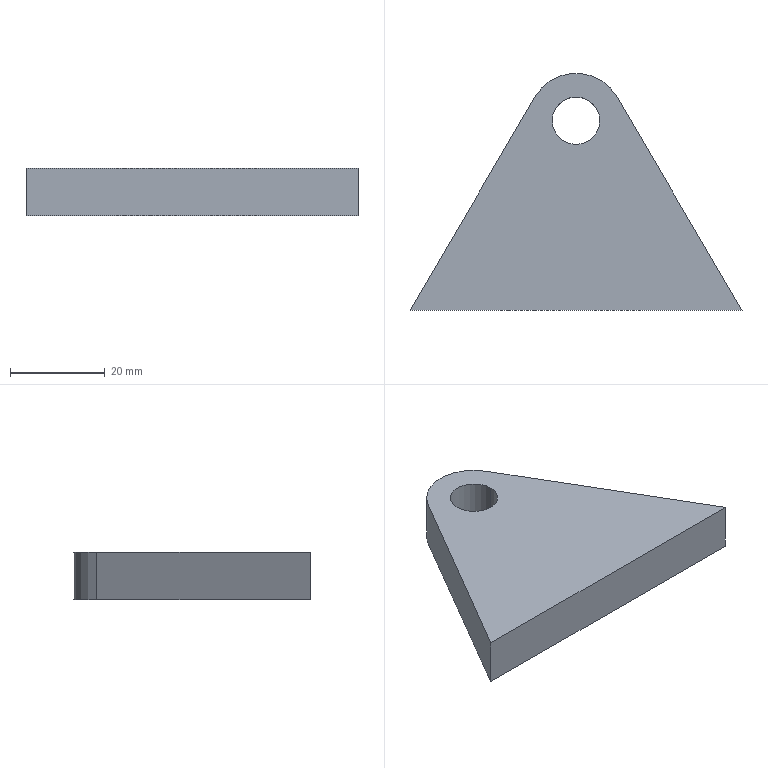Part | SolidWorks | features Extrusion 1 | 1 solid | 8 faces | box 70 x 50 x 10 mm | volume 19476 mm3 | plane 5 | cylinder 3 | commonest cylinder face diameters 10 x2 20 x1
STEP:
#1=CARTESIAN_POINT('',(-5.,0.,10.));
#2=VERTEX_POINT('',#1);
#3=CARTESIAN_POINT('',(5.,0.,10.));
#4=VERTEX_POINT('',#3);
#5=CARTESIAN_POINT('',(0.,0.,10.));
#6=DIRECTION('',(0.,0.,1.));
#7=DIRECTION('',(1.,0.,0.));
#8=AXIS2_PLACEMENT_3D('',#5,#6,#7);
#9=CIRCLE('',#8,5.);
#10=EDGE_CURVE('',#2,#4,#9,.T.);
#11=ORIENTED_EDGE('',*,*,#10,.T.);
#12=CARTESIAN_POINT('',(5.,0.,0.));
#13=VERTEX_POINT('',#12);
#14=CARTESIAN_POINT('',(5.,0.,10.));
#15=DIRECTION('',(0.,0.,-1.));
#16=VECTOR('',#15,1000.);
#17=LINE('',#14,#16);
#18=EDGE_CURVE('',#4,#13,#17,.T.);
#19=ORIENTED_EDGE('',*,*,#18,.T.);
#20=CARTESIAN_POINT('',(-5.,0.,0.));
#21=VERTEX_POINT('',#20);
#22=CARTESIAN_POINT('',(0.,0.,0.));
#23=DIRECTION('',(0.,0.,1.));
#24=DIRECTION('',(1.,0.,0.));
#25=AXIS2_PLACEMENT_3D('',#22,#23,#24);
#26=CIRCLE('',#25,5.);
#27=EDGE_CURVE('',#21,#13,#26,.T.);
#28=ORIENTED_EDGE('',*,*,#27,.F.);
#29=CARTESIAN_POINT('',(-5.,0.,10.));
#30=DIRECTION('',(0.,0.,-1.));
#31=VECTOR('',#30,1000.);
#32=LINE('',#29,#31);
#33=EDGE_CURVE('',#2,#21,#32,.T.);
#34=ORIENTED_EDGE('',*,*,#33,.F.);
#35=EDGE_LOOP('',(#11,#19,#28,#34));
#36=FACE_OUTER_BOUND('',#35,.T.);
#37=CARTESIAN_POINT('',(0.,0.,10.));
#38=DIRECTION('',(0.,0.,-1.));
#39=DIRECTION('',(-1.,0.,0.));
#40=AXIS2_PLACEMENT_3D('',#37,#38,#39);
#41=CYLINDRICAL_SURFACE('',#40,5.);
#42=ADVANCED_FACE('',(#36),#41,.F.);
#43=CARTESIAN_POINT('',(35.,-40.,10.));
#44=VERTEX_POINT('',#43);
#45=CARTESIAN_POINT('',(8.63,5.052,10.));
#46=VERTEX_POINT('',#45);
#47=CARTESIAN_POINT('',(35.,-40.,10.));
#48=DIRECTION('',(-0.5052,0.863,0.));
#49=VECTOR('',#48,1000.);
#50=LINE('',#47,#49);
#51=EDGE_CURVE('',#44,#46,#50,.T.);
#52=ORIENTED_EDGE('',*,*,#51,.T.);
#53=CARTESIAN_POINT('',(-8.63,5.052,10.));
#54=VERTEX_POINT('',#53);
#55=CARTESIAN_POINT('',(0.,0.,10.));
#56=DIRECTION('',(0.,0.,1.));
#57=DIRECTION('',(1.,0.,0.));
#58=AXIS2_PLACEMENT_3D('',#55,#56,#57);
#59=CIRCLE('',#58,10.);
#60=EDGE_CURVE('',#46,#54,#59,.T.);
#61=ORIENTED_EDGE('',*,*,#60,.T.);
#62=CARTESIAN_POINT('',(-35.,-40.,10.));
#63=VERTEX_POINT('',#62);
#64=CARTESIAN_POINT('',(-35.,-40.,10.));
#65=DIRECTION('',(-0.5052,-0.863,0.));
#66=VECTOR('',#65,1000.);
#67=LINE('',#64,#66);
#68=EDGE_CURVE('',#54,#63,#67,.T.);
#69=ORIENTED_EDGE('',*,*,#68,.T.);
#70=CARTESIAN_POINT('',(-35.,-40.,10.));
#71=DIRECTION('',(1.,0.,0.));
#72=VECTOR('',#71,1000.);
#73=LINE('',#70,#72);
#74=EDGE_CURVE('',#63,#44,#73,.T.);
#75=ORIENTED_EDGE('',*,*,#74,.T.);
#76=EDGE_LOOP('',(#52,#61,#69,#75));
#77=FACE_OUTER_BOUND('',#76,.T.);
#78=ORIENTED_EDGE('',*,*,#10,.F.);
#79=CARTESIAN_POINT('',(0.,0.,10.));
#80=DIRECTION('',(0.,0.,1.));
#81=DIRECTION('',(1.,0.,0.));
#82=AXIS2_PLACEMENT_3D('',#79,#80,#81);
#83=CIRCLE('',#82,5.);
#84=EDGE_CURVE('',#4,#2,#83,.T.);
#85=ORIENTED_EDGE('',*,*,#84,.F.);
#86=EDGE_LOOP('',(#78,#85));
#87=FACE_BOUND('',#86,.T.);
#88=CARTESIAN_POINT('',(0.,0.,10.));
#89=DIRECTION('',(0.,0.,1.));
#90=DIRECTION('',(1.,0.,0.));
#91=AXIS2_PLACEMENT_3D('',#88,#89,#90);
#92=PLANE('',#91);
#93=ADVANCED_FACE('',(#77,#87),#92,.T.);
#94=CARTESIAN_POINT('',(35.,-40.,0.));
#95=VERTEX_POINT('',#94);
#96=CARTESIAN_POINT('',(8.63,5.052,0.));
#97=VERTEX_POINT('',#96);
#98=CARTESIAN_POINT('',(35.,-40.,0.));
#99=DIRECTION('',(-0.5052,0.863,0.));
#100=VECTOR('',#99,1000.);
#101=LINE('',#98,#100);
#102=EDGE_CURVE('',#95,#97,#101,.T.);
#103=ORIENTED_EDGE('',*,*,#102,.F.);
#104=CARTESIAN_POINT('',(-35.,-40.,0.));
#105=VERTEX_POINT('',#104);
#106=CARTESIAN_POINT('',(-35.,-40.,0.));
#107=DIRECTION('',(1.,0.,0.));
#108=VECTOR('',#107,1000.);
#109=LINE('',#106,#108);
#110=EDGE_CURVE('',#105,#95,#109,.T.);
#111=ORIENTED_EDGE('',*,*,#110,.F.);
#112=CARTESIAN_POINT('',(-8.63,5.052,0.));
#113=VERTEX_POINT('',#112);
#114=CARTESIAN_POINT('',(-35.,-40.,0.));
#115=DIRECTION('',(-0.5052,-0.863,0.));
#116=VECTOR('',#115,1000.);
#117=LINE('',#114,#116);
#118=EDGE_CURVE('',#113,#105,#117,.T.);
#119=ORIENTED_EDGE('',*,*,#118,.F.);
#120=CARTESIAN_POINT('',(0.,0.,0.));
#121=DIRECTION('',(0.,0.,1.));
#122=DIRECTION('',(1.,0.,0.));
#123=AXIS2_PLACEMENT_3D('',#120,#121,#122);
#124=CIRCLE('',#123,10.);
#125=EDGE_CURVE('',#97,#113,#124,.T.);
#126=ORIENTED_EDGE('',*,*,#125,.F.);
#127=EDGE_LOOP('',(#103,#111,#119,#126));
#128=FACE_OUTER_BOUND('',#127,.T.);
#129=ORIENTED_EDGE('',*,*,#27,.T.);
#130=CARTESIAN_POINT('',(0.,0.,0.));
#131=DIRECTION('',(0.,0.,1.));
#132=DIRECTION('',(1.,0.,0.));
#133=AXIS2_PLACEMENT_3D('',#130,#131,#132);
#134=CIRCLE('',#133,5.);
#135=EDGE_CURVE('',#13,#21,#134,.T.);
#136=ORIENTED_EDGE('',*,*,#135,.T.);
#137=EDGE_LOOP('',(#129,#136));
#138=FACE_BOUND('',#137,.T.);
#139=CARTESIAN_POINT('',(0.,0.,0.));
#140=DIRECTION('',(0.,0.,1.));
#141=DIRECTION('',(1.,0.,0.));
#142=AXIS2_PLACEMENT_3D('',#139,#140,#141);
#143=PLANE('',#142);
#144=ADVANCED_FACE('',(#128,#138),#143,.F.);
#145=ORIENTED_EDGE('',*,*,#102,.T.);
#146=CARTESIAN_POINT('',(8.63,5.052,10.));
#147=DIRECTION('',(0.,0.,-1.));
#148=VECTOR('',#147,1000.);
#149=LINE('',#146,#148);
#150=EDGE_CURVE('',#46,#97,#149,.T.);
#151=ORIENTED_EDGE('',*,*,#150,.F.);
#152=ORIENTED_EDGE('',*,*,#51,.F.);
#153=CARTESIAN_POINT('',(35.,-40.,10.));
#154=DIRECTION('',(0.,0.,-1.));
#155=VECTOR('',#154,1000.);
#156=LINE('',#153,#155);
#157=EDGE_CURVE('',#44,#95,#156,.T.);
#158=ORIENTED_EDGE('',*,*,#157,.T.);
#159=EDGE_LOOP('',(#145,#151,#152,#158));
#160=FACE_OUTER_BOUND('',#159,.T.);
#161=CARTESIAN_POINT('',(35.,-40.,10.));
#162=DIRECTION('',(-0.863,-0.5052,0.));
#163=DIRECTION('',(0.5052,-0.863,0.));
#164=AXIS2_PLACEMENT_3D('',#161,#162,#163);
#165=PLANE('',#164);
#166=ADVANCED_FACE('',(#160),#165,.F.);
#167=ORIENTED_EDGE('',*,*,#125,.T.);
#168=CARTESIAN_POINT('',(-8.63,5.052,10.));
#169=DIRECTION('',(0.,0.,-1.));
#170=VECTOR('',#169,1000.);
#171=LINE('',#168,#170);
#172=EDGE_CURVE('',#54,#113,#171,.T.);
#173=ORIENTED_EDGE('',*,*,#172,.F.);
#174=ORIENTED_EDGE('',*,*,#60,.F.);
#175=ORIENTED_EDGE('',*,*,#150,.T.);
#176=EDGE_LOOP('',(#167,#173,#174,#175));
#177=FACE_OUTER_BOUND('',#176,.T.);
#178=CARTESIAN_POINT('',(0.,0.,10.));
#179=DIRECTION('',(0.,0.,-1.));
#180=DIRECTION('',(-1.,0.,0.));
#181=AXIS2_PLACEMENT_3D('',#178,#179,#180);
#182=CYLINDRICAL_SURFACE('',#181,10.);
#183=ADVANCED_FACE('',(#177),#182,.T.);
#184=ORIENTED_EDGE('',*,*,#118,.T.);
#185=CARTESIAN_POINT('',(-35.,-40.,10.));
#186=DIRECTION('',(0.,0.,-1.));
#187=VECTOR('',#186,1000.);
#188=LINE('',#185,#187);
#189=EDGE_CURVE('',#63,#105,#188,.T.);
#190=ORIENTED_EDGE('',*,*,#189,.F.);
#191=ORIENTED_EDGE('',*,*,#68,.F.);
#192=ORIENTED_EDGE('',*,*,#172,.T.);
#193=EDGE_LOOP('',(#184,#190,#191,#192));
#194=FACE_OUTER_BOUND('',#193,.T.);
#195=CARTESIAN_POINT('',(-35.,-40.,10.));
#196=DIRECTION('',(0.863,-0.5052,0.));
#197=DIRECTION('',(0.5052,0.863,0.));
#198=AXIS2_PLACEMENT_3D('',#195,#196,#197);
#199=PLANE('',#198);
#200=ADVANCED_FACE('',(#194),#199,.F.);
#201=ORIENTED_EDGE('',*,*,#110,.T.);
#202=ORIENTED_EDGE('',*,*,#157,.F.);
#203=ORIENTED_EDGE('',*,*,#74,.F.);
#204=ORIENTED_EDGE('',*,*,#189,.T.);
#205=EDGE_LOOP('',(#201,#202,#203,#204));
#206=FACE_OUTER_BOUND('',#205,.T.);
#207=CARTESIAN_POINT('',(-35.,-40.,10.));
#208=DIRECTION('',(0.,1.,0.));
#209=DIRECTION('',(-1.,0.,0.));
#210=AXIS2_PLACEMENT_3D('',#207,#208,#209);
#211=PLANE('',#210);
#212=ADVANCED_FACE('',(#206),#211,.F.);
#213=ORIENTED_EDGE('',*,*,#18,.F.);
#214=ORIENTED_EDGE('',*,*,#84,.T.);
#215=ORIENTED_EDGE('',*,*,#33,.T.);
#216=ORIENTED_EDGE('',*,*,#135,.F.);
#217=EDGE_LOOP('',(#213,#214,#215,#216));
#218=FACE_OUTER_BOUND('',#217,.T.);
#219=CARTESIAN_POINT('',(0.,0.,10.));
#220=DIRECTION('',(0.,0.,-1.));
#221=DIRECTION('',(-1.,0.,0.));
#222=AXIS2_PLACEMENT_3D('',#219,#220,#221);
#223=CYLINDRICAL_SURFACE('',#222,5.);
#224=ADVANCED_FACE('',(#218),#223,.F.);
#225=CLOSED_SHELL('',(#42,#93,#144,#166,#183,#200,#212,#224));
#226=MANIFOLD_SOLID_BREP('',#225);
#227=CARTESIAN_POINT('',(0.,0.,0.));
#228=DIRECTION('',(0.,0.,1.));
#229=DIRECTION('',(1.,0.,0.));
#230=AXIS2_PLACEMENT_3D('',#227,#228,#229);
#231=(LENGTH_UNIT()NAMED_UNIT(*)SI_UNIT(.MILLI.,.METRE.));
#232=UNCERTAINTY_MEASURE_WITH_UNIT(LENGTH_MEASURE(0.00001),#231,'','');
#233=(NAMED_UNIT(*)PLANE_ANGLE_UNIT()SI_UNIT($,.RADIAN.));
#234=(NAMED_UNIT(*)SI_UNIT($,.STERADIAN.)SOLID_ANGLE_UNIT());
#235=(GEOMETRIC_REPRESENTATION_CONTEXT(3)GLOBAL_UNCERTAINTY_ASSIGNED_CONTEXT((#232))GLOBAL_UNIT_ASSIGNED_CONTEXT((#231,#233,#234))REPRESENTATION_CONTEXT('',''));
#236=ADVANCED_BREP_SHAPE_REPRESENTATION('',(#226,#230),#235);